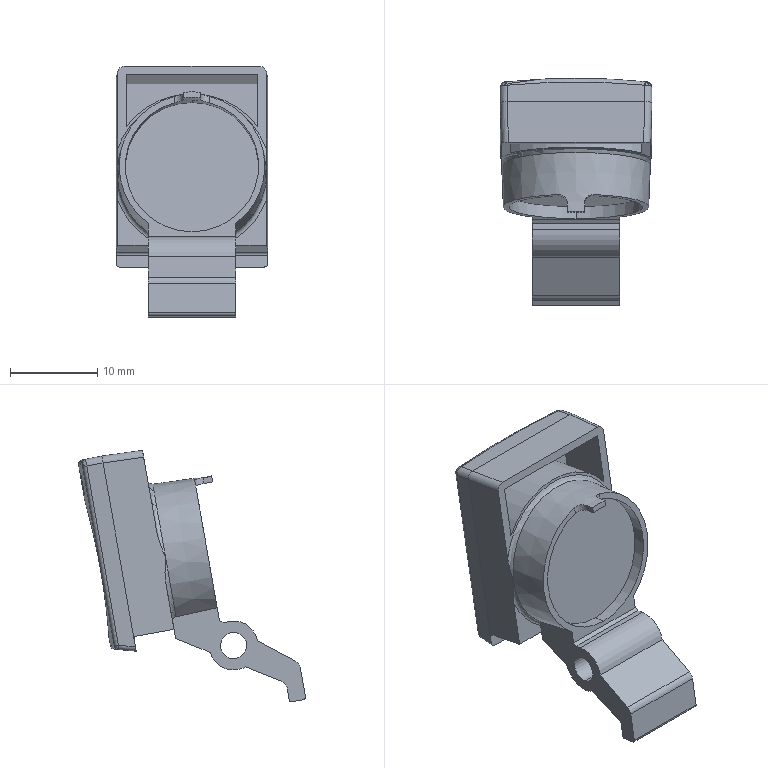Part | STEP file | _X2_751F4E45_X0_MS731-1_X2_8_27 | 1 solid | 203 faces | box 17.4 x 26.019 x 28.81 mm | volume 2994 mm3 | plane 152 | cylinder 31 | spline 12 | torus 5 | sphere 2 | cone 1 | commonest cylinder face diameters 1 x4 1.6 x4 2 x4 159.6 x4 0.6 x3 3 x2